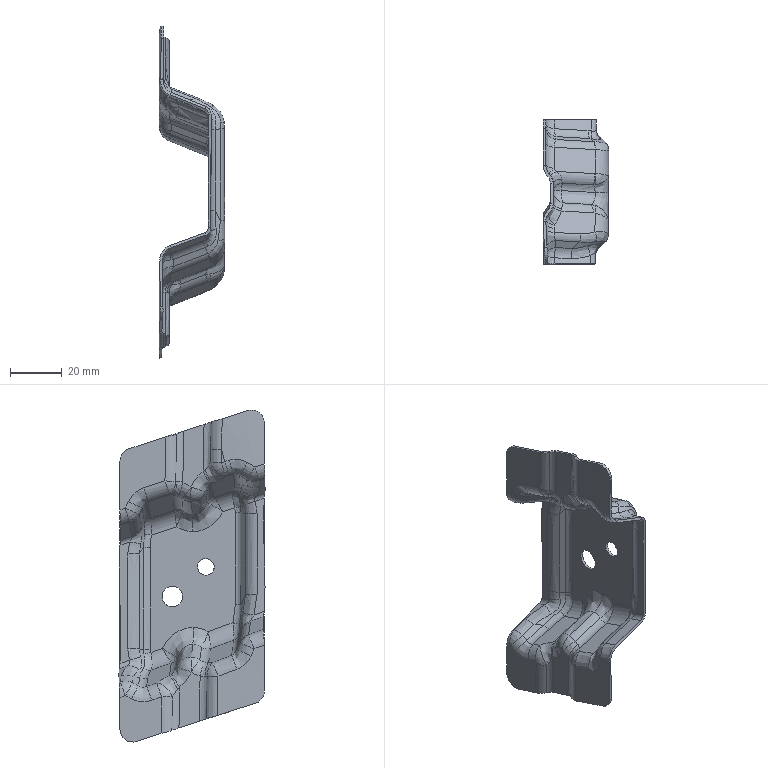Part | 1 solid | 326 faces | box 25.442 x 56.874 x 128.864 mm | volume 8344 mm3 | spline 220 | cylinder 72 | plane 18 | sphere 16 | commonest cylinder face diameters 10 x18 8 x11 12 x10 6 x7 4 x4 14 x4